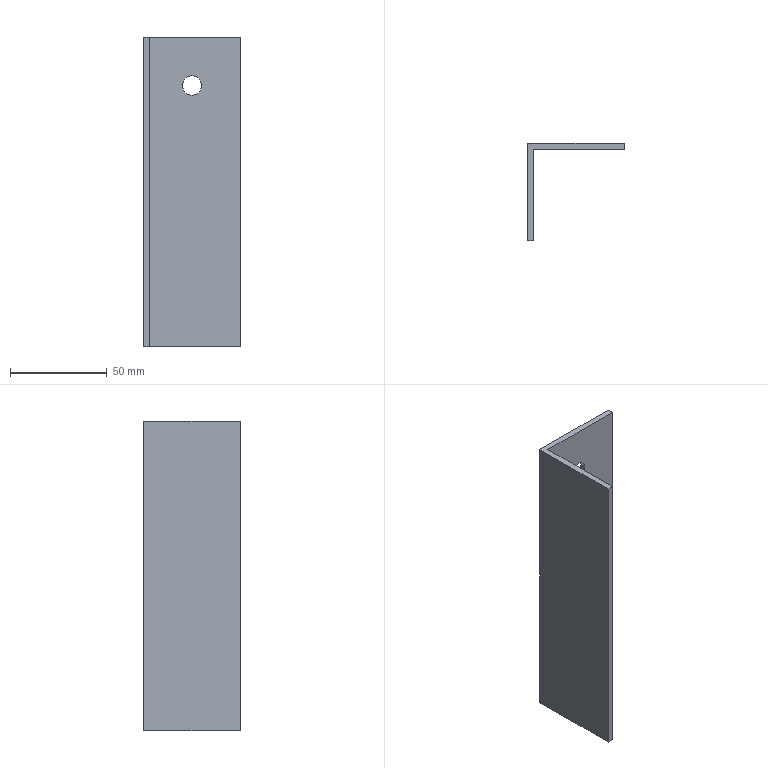Part | SolidWorks | features Extrusion 1, ICE 1 | 1 solid | 10 faces | box 50 x 50 x 160 mm | volume 46324 mm3 | plane 8 | cylinder 2 | commonest cylinder face diameters 10 x2
STEP:
#1=CARTESIAN_POINT('',(-20.,-3.,135.));
#2=VERTEX_POINT('',#1);
#3=CARTESIAN_POINT('',(-30.,-3.,135.));
#4=VERTEX_POINT('',#3);
#5=CARTESIAN_POINT('',(-25.,-3.,135.));
#6=DIRECTION('',(0.,1.,0.));
#7=DIRECTION('',(0.,0.,1.));
#8=AXIS2_PLACEMENT_3D('',#5,#6,#7);
#9=CIRCLE('',#8,5.);
#10=EDGE_CURVE('',#2,#4,#9,.T.);
#11=ORIENTED_EDGE('',*,*,#10,.F.);
#12=CARTESIAN_POINT('',(-20.,0.,135.));
#13=VERTEX_POINT('',#12);
#14=CARTESIAN_POINT('',(-20.,-10.,135.));
#15=DIRECTION('',(0.,1.,0.));
#16=VECTOR('',#15,1000.);
#17=LINE('',#14,#16);
#18=EDGE_CURVE('',#2,#13,#17,.T.);
#19=ORIENTED_EDGE('',*,*,#18,.T.);
#20=CARTESIAN_POINT('',(-30.,0.,135.));
#21=VERTEX_POINT('',#20);
#22=CARTESIAN_POINT('',(-25.,0.,135.));
#23=DIRECTION('',(0.,1.,0.));
#24=DIRECTION('',(-1.,0.,0.));
#25=AXIS2_PLACEMENT_3D('',#22,#23,#24);
#26=CIRCLE('',#25,5.);
#27=EDGE_CURVE('',#13,#21,#26,.T.);
#28=ORIENTED_EDGE('',*,*,#27,.T.);
#29=CARTESIAN_POINT('',(-30.,-10.,135.));
#30=DIRECTION('',(0.,1.,0.));
#31=VECTOR('',#30,1000.);
#32=LINE('',#29,#31);
#33=EDGE_CURVE('',#4,#21,#32,.T.);
#34=ORIENTED_EDGE('',*,*,#33,.F.);
#35=EDGE_LOOP('',(#11,#19,#28,#34));
#36=FACE_OUTER_BOUND('',#35,.T.);
#37=CARTESIAN_POINT('',(-25.,-10.,135.));
#38=DIRECTION('',(0.,1.,0.));
#39=DIRECTION('',(-1.,0.,0.));
#40=AXIS2_PLACEMENT_3D('',#37,#38,#39);
#41=CYLINDRICAL_SURFACE('',#40,5.);
#42=ADVANCED_FACE('',(#36),#41,.F.);
#43=CARTESIAN_POINT('',(0.,-3.,0.));
#44=VERTEX_POINT('',#43);
#45=CARTESIAN_POINT('',(0.,0.,0.));
#46=VERTEX_POINT('',#45);
#47=CARTESIAN_POINT('',(0.,-3.,0.));
#48=DIRECTION('',(0.,1.,0.));
#49=VECTOR('',#48,1000.);
#50=LINE('',#47,#49);
#51=EDGE_CURVE('',#44,#46,#50,.T.);
#52=ORIENTED_EDGE('',*,*,#51,.T.);
#53=CARTESIAN_POINT('',(0.,0.,160.));
#54=VERTEX_POINT('',#53);
#55=CARTESIAN_POINT('',(0.,0.,160.));
#56=DIRECTION('',(0.,0.,-1.));
#57=VECTOR('',#56,1000.);
#58=LINE('',#55,#57);
#59=EDGE_CURVE('',#54,#46,#58,.T.);
#60=ORIENTED_EDGE('',*,*,#59,.F.);
#61=CARTESIAN_POINT('',(0.,-3.,160.));
#62=VERTEX_POINT('',#61);
#63=CARTESIAN_POINT('',(0.,-3.,160.));
#64=DIRECTION('',(0.,1.,0.));
#65=VECTOR('',#64,1000.);
#66=LINE('',#63,#65);
#67=EDGE_CURVE('',#62,#54,#66,.T.);
#68=ORIENTED_EDGE('',*,*,#67,.F.);
#69=CARTESIAN_POINT('',(0.,-3.,160.));
#70=DIRECTION('',(0.,0.,-1.));
#71=VECTOR('',#70,1000.);
#72=LINE('',#69,#71);
#73=EDGE_CURVE('',#62,#44,#72,.T.);
#74=ORIENTED_EDGE('',*,*,#73,.T.);
#75=EDGE_LOOP('',(#52,#60,#68,#74));
#76=FACE_OUTER_BOUND('',#75,.T.);
#77=CARTESIAN_POINT('',(0.,-3.,160.));
#78=DIRECTION('',(-1.,0.,0.));
#79=DIRECTION('',(0.,0.,1.));
#80=AXIS2_PLACEMENT_3D('',#77,#78,#79);
#81=PLANE('',#80);
#82=ADVANCED_FACE('',(#76),#81,.F.);
#83=CARTESIAN_POINT('',(-25.,0.,135.));
#84=DIRECTION('',(0.,1.,0.));
#85=DIRECTION('',(-1.,0.,0.));
#86=AXIS2_PLACEMENT_3D('',#83,#84,#85);
#87=CIRCLE('',#86,5.);
#88=EDGE_CURVE('',#21,#13,#87,.T.);
#89=ORIENTED_EDGE('',*,*,#88,.F.);
#90=ORIENTED_EDGE('',*,*,#27,.F.);
#91=EDGE_LOOP('',(#89,#90));
#92=FACE_BOUND('',#91,.T.);
#93=CARTESIAN_POINT('',(-50.,0.,0.));
#94=VERTEX_POINT('',#93);
#95=CARTESIAN_POINT('',(0.,0.,0.));
#96=DIRECTION('',(-1.,0.,0.));
#97=VECTOR('',#96,1000.);
#98=LINE('',#95,#97);
#99=EDGE_CURVE('',#46,#94,#98,.T.);
#100=ORIENTED_EDGE('',*,*,#99,.T.);
#101=CARTESIAN_POINT('',(-50.,0.,160.));
#102=VERTEX_POINT('',#101);
#103=CARTESIAN_POINT('',(-50.,0.,160.));
#104=DIRECTION('',(0.,0.,-1.));
#105=VECTOR('',#104,1000.);
#106=LINE('',#103,#105);
#107=EDGE_CURVE('',#102,#94,#106,.T.);
#108=ORIENTED_EDGE('',*,*,#107,.F.);
#109=CARTESIAN_POINT('',(0.,0.,160.));
#110=DIRECTION('',(-1.,0.,0.));
#111=VECTOR('',#110,1000.);
#112=LINE('',#109,#111);
#113=EDGE_CURVE('',#54,#102,#112,.T.);
#114=ORIENTED_EDGE('',*,*,#113,.F.);
#115=ORIENTED_EDGE('',*,*,#59,.T.);
#116=EDGE_LOOP('',(#100,#108,#114,#115));
#117=FACE_OUTER_BOUND('',#116,.T.);
#118=CARTESIAN_POINT('',(0.,0.,160.));
#119=DIRECTION('',(0.,-1.,0.));
#120=DIRECTION('',(1.,0.,0.));
#121=AXIS2_PLACEMENT_3D('',#118,#119,#120);
#122=PLANE('',#121);
#123=ADVANCED_FACE('',(#92,#117),#122,.F.);
#124=CARTESIAN_POINT('',(-50.,-50.,0.));
#125=VERTEX_POINT('',#124);
#126=CARTESIAN_POINT('',(-50.,0.,0.));
#127=DIRECTION('',(0.,-1.,0.));
#128=VECTOR('',#127,1000.);
#129=LINE('',#126,#128);
#130=EDGE_CURVE('',#94,#125,#129,.T.);
#131=ORIENTED_EDGE('',*,*,#130,.T.);
#132=CARTESIAN_POINT('',(-50.,-50.,160.));
#133=VERTEX_POINT('',#132);
#134=CARTESIAN_POINT('',(-50.,-50.,160.));
#135=DIRECTION('',(0.,0.,-1.));
#136=VECTOR('',#135,1000.);
#137=LINE('',#134,#136);
#138=EDGE_CURVE('',#133,#125,#137,.T.);
#139=ORIENTED_EDGE('',*,*,#138,.F.);
#140=CARTESIAN_POINT('',(-50.,0.,160.));
#141=DIRECTION('',(0.,-1.,0.));
#142=VECTOR('',#141,1000.);
#143=LINE('',#140,#142);
#144=EDGE_CURVE('',#102,#133,#143,.T.);
#145=ORIENTED_EDGE('',*,*,#144,.F.);
#146=ORIENTED_EDGE('',*,*,#107,.T.);
#147=EDGE_LOOP('',(#131,#139,#145,#146));
#148=FACE_OUTER_BOUND('',#147,.T.);
#149=CARTESIAN_POINT('',(-50.,0.,160.));
#150=DIRECTION('',(1.,0.,0.));
#151=DIRECTION('',(0.,1.,0.));
#152=AXIS2_PLACEMENT_3D('',#149,#150,#151);
#153=PLANE('',#152);
#154=ADVANCED_FACE('',(#148),#153,.F.);
#155=CARTESIAN_POINT('',(-47.,-50.,0.));
#156=VERTEX_POINT('',#155);
#157=CARTESIAN_POINT('',(-50.,-50.,0.));
#158=DIRECTION('',(1.,0.,0.));
#159=VECTOR('',#158,1000.);
#160=LINE('',#157,#159);
#161=EDGE_CURVE('',#125,#156,#160,.T.);
#162=ORIENTED_EDGE('',*,*,#161,.T.);
#163=CARTESIAN_POINT('',(-47.,-50.,160.));
#164=VERTEX_POINT('',#163);
#165=CARTESIAN_POINT('',(-47.,-50.,160.));
#166=DIRECTION('',(0.,0.,-1.));
#167=VECTOR('',#166,1000.);
#168=LINE('',#165,#167);
#169=EDGE_CURVE('',#164,#156,#168,.T.);
#170=ORIENTED_EDGE('',*,*,#169,.F.);
#171=CARTESIAN_POINT('',(-50.,-50.,160.));
#172=DIRECTION('',(1.,0.,0.));
#173=VECTOR('',#172,1000.);
#174=LINE('',#171,#173);
#175=EDGE_CURVE('',#133,#164,#174,.T.);
#176=ORIENTED_EDGE('',*,*,#175,.F.);
#177=ORIENTED_EDGE('',*,*,#138,.T.);
#178=EDGE_LOOP('',(#162,#170,#176,#177));
#179=FACE_OUTER_BOUND('',#178,.T.);
#180=CARTESIAN_POINT('',(-50.,-50.,160.));
#181=DIRECTION('',(0.,1.,0.));
#182=DIRECTION('',(0.,0.,1.));
#183=AXIS2_PLACEMENT_3D('',#180,#181,#182);
#184=PLANE('',#183);
#185=ADVANCED_FACE('',(#179),#184,.F.);
#186=CARTESIAN_POINT('',(-47.,-3.,0.));
#187=VERTEX_POINT('',#186);
#188=CARTESIAN_POINT('',(-47.,-3.,0.));
#189=DIRECTION('',(0.,1.,0.));
#190=VECTOR('',#189,1000.);
#191=LINE('',#188,#190);
#192=EDGE_CURVE('',#156,#187,#191,.T.);
#193=ORIENTED_EDGE('',*,*,#192,.T.);
#194=CARTESIAN_POINT('',(-47.,-3.,160.));
#195=VERTEX_POINT('',#194);
#196=CARTESIAN_POINT('',(-47.,-3.,160.));
#197=DIRECTION('',(0.,0.,-1.));
#198=VECTOR('',#197,1000.);
#199=LINE('',#196,#198);
#200=EDGE_CURVE('',#195,#187,#199,.T.);
#201=ORIENTED_EDGE('',*,*,#200,.F.);
#202=CARTESIAN_POINT('',(-47.,-3.,160.));
#203=DIRECTION('',(0.,1.,0.));
#204=VECTOR('',#203,1000.);
#205=LINE('',#202,#204);
#206=EDGE_CURVE('',#164,#195,#205,.T.);
#207=ORIENTED_EDGE('',*,*,#206,.F.);
#208=ORIENTED_EDGE('',*,*,#169,.T.);
#209=EDGE_LOOP('',(#193,#201,#207,#208));
#210=FACE_OUTER_BOUND('',#209,.T.);
#211=CARTESIAN_POINT('',(-47.,-3.,160.));
#212=DIRECTION('',(-1.,0.,0.));
#213=DIRECTION('',(0.,0.,1.));
#214=AXIS2_PLACEMENT_3D('',#211,#212,#213);
#215=PLANE('',#214);
#216=ADVANCED_FACE('',(#210),#215,.F.);
#217=CARTESIAN_POINT('',(-25.,-3.,135.));
#218=DIRECTION('',(0.,1.,0.));
#219=DIRECTION('',(0.,0.,1.));
#220=AXIS2_PLACEMENT_3D('',#217,#218,#219);
#221=CIRCLE('',#220,5.);
#222=EDGE_CURVE('',#4,#2,#221,.T.);
#223=ORIENTED_EDGE('',*,*,#222,.T.);
#224=ORIENTED_EDGE('',*,*,#10,.T.);
#225=EDGE_LOOP('',(#223,#224));
#226=FACE_BOUND('',#225,.T.);
#227=CARTESIAN_POINT('',(0.,-3.,0.));
#228=DIRECTION('',(1.,0.,0.));
#229=VECTOR('',#228,1000.);
#230=LINE('',#227,#229);
#231=EDGE_CURVE('',#187,#44,#230,.T.);
#232=ORIENTED_EDGE('',*,*,#231,.T.);
#233=ORIENTED_EDGE('',*,*,#73,.F.);
#234=CARTESIAN_POINT('',(0.,-3.,160.));
#235=DIRECTION('',(1.,0.,0.));
#236=VECTOR('',#235,1000.);
#237=LINE('',#234,#236);
#238=EDGE_CURVE('',#195,#62,#237,.T.);
#239=ORIENTED_EDGE('',*,*,#238,.F.);
#240=ORIENTED_EDGE('',*,*,#200,.T.);
#241=EDGE_LOOP('',(#232,#233,#239,#240));
#242=FACE_OUTER_BOUND('',#241,.T.);
#243=CARTESIAN_POINT('',(0.,-3.,160.));
#244=DIRECTION('',(0.,1.,0.));
#245=DIRECTION('',(0.,0.,1.));
#246=AXIS2_PLACEMENT_3D('',#243,#244,#245);
#247=PLANE('',#246);
#248=ADVANCED_FACE('',(#226,#242),#247,.F.);
#249=ORIENTED_EDGE('',*,*,#67,.T.);
#250=ORIENTED_EDGE('',*,*,#113,.T.);
#251=ORIENTED_EDGE('',*,*,#144,.T.);
#252=ORIENTED_EDGE('',*,*,#175,.T.);
#253=ORIENTED_EDGE('',*,*,#206,.T.);
#254=ORIENTED_EDGE('',*,*,#238,.T.);
#255=EDGE_LOOP('',(#249,#250,#251,#252,#253,#254));
#256=FACE_OUTER_BOUND('',#255,.T.);
#257=CARTESIAN_POINT('',(0.,0.,160.));
#258=DIRECTION('',(0.,0.,1.));
#259=DIRECTION('',(1.,0.,0.));
#260=AXIS2_PLACEMENT_3D('',#257,#258,#259);
#261=PLANE('',#260);
#262=ADVANCED_FACE('',(#256),#261,.T.);
#263=ORIENTED_EDGE('',*,*,#51,.F.);
#264=ORIENTED_EDGE('',*,*,#231,.F.);
#265=ORIENTED_EDGE('',*,*,#192,.F.);
#266=ORIENTED_EDGE('',*,*,#161,.F.);
#267=ORIENTED_EDGE('',*,*,#130,.F.);
#268=ORIENTED_EDGE('',*,*,#99,.F.);
#269=EDGE_LOOP('',(#263,#264,#265,#266,#267,#268));
#270=FACE_OUTER_BOUND('',#269,.T.);
#271=CARTESIAN_POINT('',(0.,0.,0.));
#272=DIRECTION('',(0.,0.,1.));
#273=DIRECTION('',(1.,0.,0.));
#274=AXIS2_PLACEMENT_3D('',#271,#272,#273);
#275=PLANE('',#274);
#276=ADVANCED_FACE('',(#270),#275,.F.);
#277=ORIENTED_EDGE('',*,*,#18,.F.);
#278=ORIENTED_EDGE('',*,*,#222,.F.);
#279=ORIENTED_EDGE('',*,*,#33,.T.);
#280=ORIENTED_EDGE('',*,*,#88,.T.);
#281=EDGE_LOOP('',(#277,#278,#279,#280));
#282=FACE_OUTER_BOUND('',#281,.T.);
#283=CARTESIAN_POINT('',(-25.,-10.,135.));
#284=DIRECTION('',(0.,1.,0.));
#285=DIRECTION('',(-1.,0.,0.));
#286=AXIS2_PLACEMENT_3D('',#283,#284,#285);
#287=CYLINDRICAL_SURFACE('',#286,5.);
#288=ADVANCED_FACE('',(#282),#287,.F.);
#289=CLOSED_SHELL('',(#42,#82,#123,#154,#185,#216,#248,#262,#276,#288));
#290=MANIFOLD_SOLID_BREP('',#289);
#291=CARTESIAN_POINT('',(0.,0.,0.));
#292=DIRECTION('',(0.,0.,1.));
#293=DIRECTION('',(1.,0.,0.));
#294=AXIS2_PLACEMENT_3D('',#291,#292,#293);
#295=(LENGTH_UNIT()NAMED_UNIT(*)SI_UNIT(.MILLI.,.METRE.));
#296=UNCERTAINTY_MEASURE_WITH_UNIT(LENGTH_MEASURE(0.00001),#295,'','');
#297=(NAMED_UNIT(*)PLANE_ANGLE_UNIT()SI_UNIT($,.RADIAN.));
#298=(NAMED_UNIT(*)SI_UNIT($,.STERADIAN.)SOLID_ANGLE_UNIT());
#299=(GEOMETRIC_REPRESENTATION_CONTEXT(3)GLOBAL_UNCERTAINTY_ASSIGNED_CONTEXT((#296))GLOBAL_UNIT_ASSIGNED_CONTEXT((#295,#297,#298))REPRESENTATION_CONTEXT('',''));
#300=ADVANCED_BREP_SHAPE_REPRESENTATION('',(#290,#294),#299);